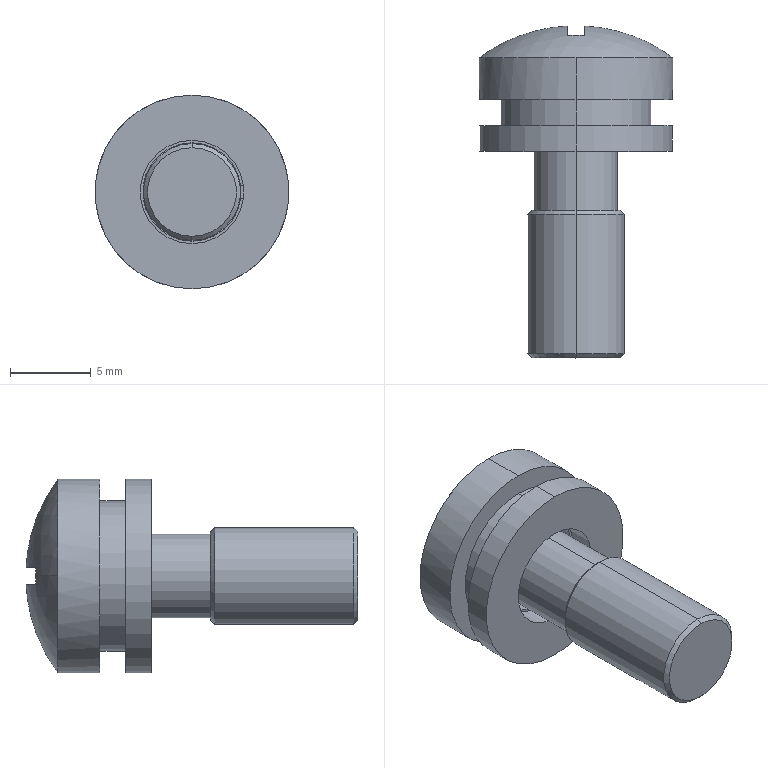Part | STEP file | 3 solids | 46 faces | box 12 x 20.569 x 12 mm | volume 958.317 mm3 | plane 22 | cylinder 16 | cone 4 | torus 2 | sphere 2 | commonest cylinder face diameters 12 x4 6.1 x3 9.3 x3 5.2 x2 6 x2 6.4 x2
STEP:
#1=CARTESIAN_POINT('',(0.,-20.6,-2.75));
#2=VERTEX_POINT('',#1);
#3=CARTESIAN_POINT('',(0.,-20.6,2.75));
#4=VERTEX_POINT('',#3);
#5=CARTESIAN_POINT('',(0.,-20.6,0.));
#6=DIRECTION('',(0.,-1.,0.));
#7=DIRECTION('',(0.,0.,1.));
#8=AXIS2_PLACEMENT_3D('',#5,#6,#7);
#9=CIRCLE('',#8,2.75);
#10=EDGE_CURVE('',#2,#4,#9,.T.);
#11=ORIENTED_EDGE('',*,*,#10,.F.);
#12=CARTESIAN_POINT('',(0.,-20.35,-3.));
#13=VERTEX_POINT('',#12);
#14=CARTESIAN_POINT('',(0.,-20.6,-2.75));
#15=DIRECTION('',(0.,0.7071,-0.7071));
#16=VECTOR('',#15,1000.);
#17=LINE('',#14,#16);
#18=EDGE_CURVE('',#2,#13,#17,.T.);
#19=ORIENTED_EDGE('',*,*,#18,.T.);
#20=CARTESIAN_POINT('',(0.,-20.35,3.));
#21=VERTEX_POINT('',#20);
#22=CARTESIAN_POINT('',(0.,-20.35,0.));
#23=DIRECTION('',(0.,1.,0.));
#24=DIRECTION('',(0.,0.,1.));
#25=AXIS2_PLACEMENT_3D('',#22,#23,#24);
#26=CIRCLE('',#25,3.);
#27=EDGE_CURVE('',#21,#13,#26,.T.);
#28=ORIENTED_EDGE('',*,*,#27,.F.);
#29=CARTESIAN_POINT('',(0.,-20.6,2.75));
#30=DIRECTION('',(0.,0.7071,0.7071));
#31=VECTOR('',#30,1000.);
#32=LINE('',#29,#31);
#33=EDGE_CURVE('',#4,#21,#32,.T.);
#34=ORIENTED_EDGE('',*,*,#33,.F.);
#35=EDGE_LOOP('',(#11,#19,#28,#34));
#36=FACE_OUTER_BOUND('',#35,.T.);
#37=CARTESIAN_POINT('',(0.,-20.6,0.));
#38=DIRECTION('',(0.,1.,0.));
#39=DIRECTION('',(0.,0.,1.));
#40=AXIS2_PLACEMENT_3D('',#37,#38,#39);
#41=CONICAL_SURFACE('',#40,2.75,0.7854);
#42=ADVANCED_FACE('',(#36),#41,.T.);
#43=CARTESIAN_POINT('',(0.,-11.46,2.75));
#44=VERTEX_POINT('',#43);
#45=CARTESIAN_POINT('',(0.,-11.46,-2.75));
#46=VERTEX_POINT('',#45);
#47=CARTESIAN_POINT('',(0.,-11.46,0.));
#48=DIRECTION('',(0.,1.,0.));
#49=DIRECTION('',(0.,0.,1.));
#50=AXIS2_PLACEMENT_3D('',#47,#48,#49);
#51=CIRCLE('',#50,2.75);
#52=EDGE_CURVE('',#44,#46,#51,.T.);
#53=ORIENTED_EDGE('',*,*,#52,.F.);
#54=CARTESIAN_POINT('',(0.,-11.71,3.));
#55=VERTEX_POINT('',#54);
#56=CARTESIAN_POINT('',(0.,-11.71,3.));
#57=DIRECTION('',(0.,-0.7071,0.7071));
#58=VECTOR('',#57,1000.);
#59=LINE('',#56,#58);
#60=EDGE_CURVE('',#44,#55,#59,.T.);
#61=ORIENTED_EDGE('',*,*,#60,.T.);
#62=CARTESIAN_POINT('',(0.,-11.71,-3.));
#63=VERTEX_POINT('',#62);
#64=CARTESIAN_POINT('',(0.,-11.71,0.));
#65=DIRECTION('',(0.,-1.,0.));
#66=DIRECTION('',(0.,0.,1.));
#67=AXIS2_PLACEMENT_3D('',#64,#65,#66);
#68=CIRCLE('',#67,3.);
#69=EDGE_CURVE('',#63,#55,#68,.T.);
#70=ORIENTED_EDGE('',*,*,#69,.F.);
#71=CARTESIAN_POINT('',(0.,-11.71,-3.));
#72=DIRECTION('',(0.,-0.7071,-0.7071));
#73=VECTOR('',#72,1000.);
#74=LINE('',#71,#73);
#75=EDGE_CURVE('',#46,#63,#74,.T.);
#76=ORIENTED_EDGE('',*,*,#75,.F.);
#77=EDGE_LOOP('',(#53,#61,#70,#76));
#78=FACE_OUTER_BOUND('',#77,.T.);
#79=CARTESIAN_POINT('',(0.,-11.71,0.));
#80=DIRECTION('',(0.,-1.,0.));
#81=DIRECTION('',(0.,0.,-1.));
#82=AXIS2_PLACEMENT_3D('',#79,#80,#81);
#83=CONICAL_SURFACE('',#82,3.,0.7854);
#84=ADVANCED_FACE('',(#78),#83,.T.);
#85=CARTESIAN_POINT('',(0.,-4.85,2.6));
#86=VERTEX_POINT('',#85);
#87=CARTESIAN_POINT('',(0.,-4.85,-2.6));
#88=VERTEX_POINT('',#87);
#89=CARTESIAN_POINT('',(0.,-4.85,0.));
#90=DIRECTION('',(0.,-1.,0.));
#91=DIRECTION('',(0.,0.,-1.));
#92=AXIS2_PLACEMENT_3D('',#89,#90,#91);
#93=CIRCLE('',#92,2.6);
#94=EDGE_CURVE('',#86,#88,#93,.T.);
#95=ORIENTED_EDGE('',*,*,#94,.F.);
#96=CARTESIAN_POINT('',(0.,-4.6,2.85));
#97=VERTEX_POINT('',#96);
#98=CARTESIAN_POINT('',(0.,-4.85,2.85));
#99=DIRECTION('',(1.,0.,0.));
#100=DIRECTION('',(0.,0.,-1.));
#101=AXIS2_PLACEMENT_3D('',#98,#99,#100);
#102=CIRCLE('',#101,0.25);
#103=EDGE_CURVE('',#86,#97,#102,.T.);
#104=ORIENTED_EDGE('',*,*,#103,.T.);
#105=CARTESIAN_POINT('',(0.,-4.6,-2.85));
#106=VERTEX_POINT('',#105);
#107=CARTESIAN_POINT('',(0.,-4.6,0.));
#108=DIRECTION('',(0.,1.,0.));
#109=DIRECTION('',(0.,0.,-1.));
#110=AXIS2_PLACEMENT_3D('',#107,#108,#109);
#111=CIRCLE('',#110,2.85);
#112=EDGE_CURVE('',#106,#97,#111,.T.);
#113=ORIENTED_EDGE('',*,*,#112,.F.);
#114=CARTESIAN_POINT('',(0.,-4.85,-2.85));
#115=DIRECTION('',(-1.,0.,0.));
#116=DIRECTION('',(0.,0.,1.));
#117=AXIS2_PLACEMENT_3D('',#114,#115,#116);
#118=CIRCLE('',#117,0.25);
#119=EDGE_CURVE('',#88,#106,#118,.T.);
#120=ORIENTED_EDGE('',*,*,#119,.F.);
#121=EDGE_LOOP('',(#95,#104,#113,#120));
#122=FACE_OUTER_BOUND('',#121,.T.);
#123=CARTESIAN_POINT('',(0.,-4.85,0.));
#124=DIRECTION('',(0.,-1.,0.));
#125=DIRECTION('',(0.,0.,-1.));
#126=AXIS2_PLACEMENT_3D('',#123,#124,#125);
#127=TOROIDAL_SURFACE('',#126,2.85,0.25);
#128=ADVANCED_FACE('',(#122),#127,.F.);
#129=CARTESIAN_POINT('',(-3.45,-0.614,0.));
#130=VERTEX_POINT('',#129);
#131=CARTESIAN_POINT('',(-3.45,-0.6304,0.555));
#132=VERTEX_POINT('',#131);
#133=CARTESIAN_POINT('',(-3.45,-10.,0.));
#134=DIRECTION('',(1.,0.,0.));
#135=DIRECTION('',(0.,0.,1.));
#136=AXIS2_PLACEMENT_3D('',#133,#134,#135);
#137=CIRCLE('',#136,9.386);
#138=EDGE_CURVE('',#130,#132,#137,.T.);
#139=ORIENTED_EDGE('',*,*,#138,.F.);
#140=CARTESIAN_POINT('',(-6.,-2.,0.));
#141=VERTEX_POINT('',#140);
#142=CARTESIAN_POINT('',(0.,-10.,0.));
#143=DIRECTION('',(0.,0.,1.));
#144=DIRECTION('',(1.,0.,0.));
#145=AXIS2_PLACEMENT_3D('',#142,#143,#144);
#146=CIRCLE('',#145,10.);
#147=EDGE_CURVE('',#130,#141,#146,.T.);
#148=ORIENTED_EDGE('',*,*,#147,.T.);
#149=CARTESIAN_POINT('',(0.,-2.,6.));
#150=VERTEX_POINT('',#149);
#151=CARTESIAN_POINT('',(0.,-2.,0.));
#152=DIRECTION('',(0.,-1.,0.));
#153=DIRECTION('',(0.,0.,-1.));
#154=AXIS2_PLACEMENT_3D('',#151,#152,#153);
#155=CIRCLE('',#154,6.);
#156=EDGE_CURVE('',#150,#141,#155,.T.);
#157=ORIENTED_EDGE('',*,*,#156,.F.);
#158=CARTESIAN_POINT('',(6.,-2.,0.));
#159=VERTEX_POINT('',#158);
#160=CARTESIAN_POINT('',(0.,-2.,0.));
#161=DIRECTION('',(0.,-1.,0.));
#162=DIRECTION('',(0.,0.,-1.));
#163=AXIS2_PLACEMENT_3D('',#160,#161,#162);
#164=CIRCLE('',#163,6.);
#165=EDGE_CURVE('',#159,#150,#164,.T.);
#166=ORIENTED_EDGE('',*,*,#165,.F.);
#167=CARTESIAN_POINT('',(3.45,-0.614,0.));
#168=VERTEX_POINT('',#167);
#169=CARTESIAN_POINT('',(0.,-10.,0.));
#170=DIRECTION('',(0.,0.,-1.));
#171=DIRECTION('',(-1.,0.,0.));
#172=AXIS2_PLACEMENT_3D('',#169,#170,#171);
#173=CIRCLE('',#172,10.);
#174=EDGE_CURVE('',#168,#159,#173,.T.);
#175=ORIENTED_EDGE('',*,*,#174,.F.);
#176=CARTESIAN_POINT('',(3.45,-0.6304,0.555));
#177=VERTEX_POINT('',#176);
#178=CARTESIAN_POINT('',(3.45,-10.,0.));
#179=DIRECTION('',(-1.,0.,0.));
#180=DIRECTION('',(0.,0.,-1.));
#181=AXIS2_PLACEMENT_3D('',#178,#179,#180);
#182=CIRCLE('',#181,9.386);
#183=EDGE_CURVE('',#177,#168,#182,.T.);
#184=ORIENTED_EDGE('',*,*,#183,.F.);
#185=CARTESIAN_POINT('',(0.555,-0.03085,0.555));
#186=VERTEX_POINT('',#185);
#187=CARTESIAN_POINT('',(0.,-10.,0.555));
#188=DIRECTION('',(0.,0.,-1.));
#189=DIRECTION('',(1.,0.,0.));
#190=AXIS2_PLACEMENT_3D('',#187,#188,#189);
#191=CIRCLE('',#190,9.985);
#192=EDGE_CURVE('',#186,#177,#191,.T.);
#193=ORIENTED_EDGE('',*,*,#192,.F.);
#194=CARTESIAN_POINT('',(0.555,-0.6304,3.45));
#195=VERTEX_POINT('',#194);
#196=CARTESIAN_POINT('',(0.555,-10.,0.));
#197=DIRECTION('',(-1.,0.,0.));
#198=DIRECTION('',(0.,0.,-1.));
#199=AXIS2_PLACEMENT_3D('',#196,#197,#198);
#200=CIRCLE('',#199,9.985);
#201=EDGE_CURVE('',#195,#186,#200,.T.);
#202=ORIENTED_EDGE('',*,*,#201,.F.);
#203=CARTESIAN_POINT('',(-0.555,-0.6304,3.45));
#204=VERTEX_POINT('',#203);
#205=CARTESIAN_POINT('',(0.,-10.,3.45));
#206=DIRECTION('',(0.,0.,-1.));
#207=DIRECTION('',(1.,0.,0.));
#208=AXIS2_PLACEMENT_3D('',#205,#206,#207);
#209=CIRCLE('',#208,9.386);
#210=EDGE_CURVE('',#204,#195,#209,.T.);
#211=ORIENTED_EDGE('',*,*,#210,.F.);
#212=CARTESIAN_POINT('',(-0.555,-0.03085,0.555));
#213=VERTEX_POINT('',#212);
#214=CARTESIAN_POINT('',(-0.555,-10.,0.));
#215=DIRECTION('',(1.,0.,0.));
#216=DIRECTION('',(0.,0.,1.));
#217=AXIS2_PLACEMENT_3D('',#214,#215,#216);
#218=CIRCLE('',#217,9.985);
#219=EDGE_CURVE('',#213,#204,#218,.T.);
#220=ORIENTED_EDGE('',*,*,#219,.F.);
#221=CARTESIAN_POINT('',(0.,-10.,0.555));
#222=DIRECTION('',(0.,0.,-1.));
#223=DIRECTION('',(1.,0.,0.));
#224=AXIS2_PLACEMENT_3D('',#221,#222,#223);
#225=CIRCLE('',#224,9.985);
#226=EDGE_CURVE('',#132,#213,#225,.T.);
#227=ORIENTED_EDGE('',*,*,#226,.F.);
#228=EDGE_LOOP('',(#139,#148,#157,#166,#175,#184,#193,#202,#211,#220,#227));
#229=FACE_OUTER_BOUND('',#228,.T.);
#230=CARTESIAN_POINT('',(0.,-10.,0.));
#231=DIRECTION('',(0.,0.,1.));
#232=DIRECTION('',(1.,0.,0.));
#233=AXIS2_PLACEMENT_3D('',#230,#231,#232);
#234=SPHERICAL_SURFACE('',#233,10.);
#235=ADVANCED_FACE('',(#229),#234,.T.);
#236=CARTESIAN_POINT('',(0.,-2.,-6.));
#237=VERTEX_POINT('',#236);
#238=CARTESIAN_POINT('',(0.,-2.,0.));
#239=DIRECTION('',(0.,-1.,0.));
#240=DIRECTION('',(0.,0.,-1.));
#241=AXIS2_PLACEMENT_3D('',#238,#239,#240);
#242=CIRCLE('',#241,6.);
#243=EDGE_CURVE('',#237,#159,#242,.T.);
#244=ORIENTED_EDGE('',*,*,#243,.T.);
#245=ORIENTED_EDGE('',*,*,#165,.T.);
#246=CARTESIAN_POINT('',(0.,-4.6,6.));
#247=VERTEX_POINT('',#246);
#248=CARTESIAN_POINT('',(0.,-20.6,6.));
#249=DIRECTION('',(0.,-1.,0.));
#250=VECTOR('',#249,1000.);
#251=LINE('',#248,#250);
#252=EDGE_CURVE('',#150,#247,#251,.T.);
#253=ORIENTED_EDGE('',*,*,#252,.T.);
#254=CARTESIAN_POINT('',(0.,-4.6,-6.));
#255=VERTEX_POINT('',#254);
#256=CARTESIAN_POINT('',(0.,-4.6,0.));
#257=DIRECTION('',(0.,-1.,0.));
#258=DIRECTION('',(0.,0.,-1.));
#259=AXIS2_PLACEMENT_3D('',#256,#257,#258);
#260=CIRCLE('',#259,6.);
#261=EDGE_CURVE('',#255,#247,#260,.T.);
#262=ORIENTED_EDGE('',*,*,#261,.F.);
#263=CARTESIAN_POINT('',(0.,-20.6,-6.));
#264=DIRECTION('',(0.,-1.,0.));
#265=VECTOR('',#264,1000.);
#266=LINE('',#263,#265);
#267=EDGE_CURVE('',#237,#255,#266,.T.);
#268=ORIENTED_EDGE('',*,*,#267,.F.);
#269=EDGE_LOOP('',(#244,#245,#253,#262,#268));
#270=FACE_OUTER_BOUND('',#269,.T.);
#271=CARTESIAN_POINT('',(0.,-20.6,0.));
#272=DIRECTION('',(0.,-1.,0.));
#273=DIRECTION('',(0.,0.,-1.));
#274=AXIS2_PLACEMENT_3D('',#271,#272,#273);
#275=CYLINDRICAL_SURFACE('',#274,6.);
#276=ADVANCED_FACE('',(#270),#275,.T.);
#277=CARTESIAN_POINT('',(0.,-4.85,0.));
#278=DIRECTION('',(0.,-1.,0.));
#279=DIRECTION('',(0.,0.,-1.));
#280=AXIS2_PLACEMENT_3D('',#277,#278,#279);
#281=CIRCLE('',#280,2.6);
#282=EDGE_CURVE('',#88,#86,#281,.T.);
#283=ORIENTED_EDGE('',*,*,#282,.T.);
#284=CARTESIAN_POINT('',(0.,-11.46,2.6));
#285=VERTEX_POINT('',#284);
#286=CARTESIAN_POINT('',(0.,-20.6,2.6));
#287=DIRECTION('',(0.,-1.,0.));
#288=VECTOR('',#287,1000.);
#289=LINE('',#286,#288);
#290=EDGE_CURVE('',#86,#285,#289,.T.);
#291=ORIENTED_EDGE('',*,*,#290,.T.);
#292=CARTESIAN_POINT('',(0.,-11.46,-2.6));
#293=VERTEX_POINT('',#292);
#294=CARTESIAN_POINT('',(0.,-11.46,0.));
#295=DIRECTION('',(0.,-1.,0.));
#296=DIRECTION('',(0.,0.,-1.));
#297=AXIS2_PLACEMENT_3D('',#294,#295,#296);
#298=CIRCLE('',#297,2.6);
#299=EDGE_CURVE('',#293,#285,#298,.T.);
#300=ORIENTED_EDGE('',*,*,#299,.F.);
#301=CARTESIAN_POINT('',(0.,-20.6,-2.6));
#302=DIRECTION('',(0.,-1.,0.));
#303=VECTOR('',#302,1000.);
#304=LINE('',#301,#303);
#305=EDGE_CURVE('',#88,#293,#304,.T.);
#306=ORIENTED_EDGE('',*,*,#305,.F.);
#307=EDGE_LOOP('',(#283,#291,#300,#306));
#308=FACE_OUTER_BOUND('',#307,.T.);
#309=CARTESIAN_POINT('',(0.,-20.6,0.));
#310=DIRECTION('',(0.,-1.,0.));
#311=DIRECTION('',(0.,0.,-1.));
#312=AXIS2_PLACEMENT_3D('',#309,#310,#311);
#313=CYLINDRICAL_SURFACE('',#312,2.6);
#314=ADVANCED_FACE('',(#308),#313,.T.);
#315=ORIENTED_EDGE('',*,*,#69,.T.);
#316=CARTESIAN_POINT('',(0.,-20.6,3.));
#317=DIRECTION('',(0.,-1.,0.));
#318=VECTOR('',#317,1000.);
#319=LINE('',#316,#318);
#320=EDGE_CURVE('',#55,#21,#319,.T.);
#321=ORIENTED_EDGE('',*,*,#320,.T.);
#322=ORIENTED_EDGE('',*,*,#27,.T.);
#323=CARTESIAN_POINT('',(0.,-20.6,-3.));
#324=DIRECTION('',(0.,-1.,0.));
#325=VECTOR('',#324,1000.);
#326=LINE('',#323,#325);
#327=EDGE_CURVE('',#63,#13,#326,.T.);
#328=ORIENTED_EDGE('',*,*,#327,.F.);
#329=EDGE_LOOP('',(#315,#321,#322,#328));
#330=FACE_OUTER_BOUND('',#329,.T.);
#331=CARTESIAN_POINT('',(0.,-20.6,0.));
#332=DIRECTION('',(0.,-1.,0.));
#333=DIRECTION('',(0.,0.,-1.));
#334=AXIS2_PLACEMENT_3D('',#331,#332,#333);
#335=CYLINDRICAL_SURFACE('',#334,3.);
#336=ADVANCED_FACE('',(#330),#335,.T.);
#337=CARTESIAN_POINT('',(0.,-20.6,0.));
#338=DIRECTION('',(0.,-1.,0.));
#339=DIRECTION('',(0.,0.,1.));
#340=AXIS2_PLACEMENT_3D('',#337,#338,#339);
#341=CIRCLE('',#340,2.75);
#342=EDGE_CURVE('',#4,#2,#341,.T.);
#343=ORIENTED_EDGE('',*,*,#342,.T.);
#344=ORIENTED_EDGE('',*,*,#10,.T.);
#345=EDGE_LOOP('',(#343,#344));
#346=FACE_OUTER_BOUND('',#345,.T.);
#347=CARTESIAN_POINT('',(0.,-20.6,0.));
#348=DIRECTION('',(0.,1.,0.));
#349=DIRECTION('',(0.,0.,1.));
#350=AXIS2_PLACEMENT_3D('',#347,#348,#349);
#351=PLANE('',#350);
#352=ADVANCED_FACE('',(#346),#351,.F.);
#353=ORIENTED_EDGE('',*,*,#320,.F.);
#354=CARTESIAN_POINT('',(0.,-11.71,0.));
#355=DIRECTION('',(0.,-1.,0.));
#356=DIRECTION('',(0.,0.,1.));
#357=AXIS2_PLACEMENT_3D('',#354,#355,#356);
#358=CIRCLE('',#357,3.);
#359=EDGE_CURVE('',#55,#63,#358,.T.);
#360=ORIENTED_EDGE('',*,*,#359,.T.);
#361=ORIENTED_EDGE('',*,*,#327,.T.);
#362=CARTESIAN_POINT('',(0.,-20.35,0.));
#363=DIRECTION('',(0.,1.,0.));
#364=DIRECTION('',(0.,0.,1.));
#365=AXIS2_PLACEMENT_3D('',#362,#363,#364);
#366=CIRCLE('',#365,3.);
#367=EDGE_CURVE('',#13,#21,#366,.T.);
#368=ORIENTED_EDGE('',*,*,#367,.T.);
#369=EDGE_LOOP('',(#353,#360,#361,#368));
#370=FACE_OUTER_BOUND('',#369,.T.);
#371=CARTESIAN_POINT('',(0.,-20.6,0.));
#372=DIRECTION('',(0.,-1.,0.));
#373=DIRECTION('',(0.,0.,-1.));
#374=AXIS2_PLACEMENT_3D('',#371,#372,#373);
#375=CYLINDRICAL_SURFACE('',#374,3.);
#376=ADVANCED_FACE('',(#370),#375,.T.);
#377=CARTESIAN_POINT('',(0.,-11.46,0.));
#378=DIRECTION('',(0.,1.,0.));
#379=DIRECTION('',(0.,0.,1.));
#380=AXIS2_PLACEMENT_3D('',#377,#378,#379);
#381=CIRCLE('',#380,2.75);
#382=EDGE_CURVE('',#46,#44,#381,.T.);
#383=ORIENTED_EDGE('',*,*,#382,.T.);
#384=ORIENTED_EDGE('',*,*,#52,.T.);
#385=EDGE_LOOP('',(#383,#384));
#386=FACE_OUTER_BOUND('',#385,.T.);
#387=ORIENTED_EDGE('',*,*,#299,.T.);
#388=CARTESIAN_POINT('',(0.,-11.46,0.));
#389=DIRECTION('',(0.,-1.,0.));
#390=DIRECTION('',(0.,0.,-1.));
#391=AXIS2_PLACEMENT_3D('',#388,#389,#390);
#392=CIRCLE('',#391,2.6);
#393=EDGE_CURVE('',#285,#293,#392,.T.);
#394=ORIENTED_EDGE('',*,*,#393,.T.);
#395=EDGE_LOOP('',(#387,#394));
#396=FACE_BOUND('',#395,.T.);
#397=CARTESIAN_POINT('',(0.,-11.46,0.));
#398=DIRECTION('',(0.,1.,0.));
#399=DIRECTION('',(0.,0.,1.));
#400=AXIS2_PLACEMENT_3D('',#397,#398,#399);
#401=PLANE('',#400);
#402=ADVANCED_FACE('',(#386,#396),#401,.T.);
#403=ORIENTED_EDGE('',*,*,#290,.F.);
#404=ORIENTED_EDGE('',*,*,#94,.T.);
#405=ORIENTED_EDGE('',*,*,#305,.T.);
#406=ORIENTED_EDGE('',*,*,#393,.F.);
#407=EDGE_LOOP('',(#403,#404,#405,#406));
#408=FACE_OUTER_BOUND('',#407,.T.);
#409=CARTESIAN_POINT('',(0.,-20.6,0.));
#410=DIRECTION('',(0.,-1.,0.));
#411=DIRECTION('',(0.,0.,-1.));
#412=AXIS2_PLACEMENT_3D('',#409,#410,#411);
#413=CYLINDRICAL_SURFACE('',#412,2.6);
#414=ADVANCED_FACE('',(#408),#413,.T.);
#415=ORIENTED_EDGE('',*,*,#112,.T.);
#416=CARTESIAN_POINT('',(0.,-4.6,0.));
#417=DIRECTION('',(0.,1.,0.));
#418=DIRECTION('',(0.,0.,-1.));
#419=AXIS2_PLACEMENT_3D('',#416,#417,#418);
#420=CIRCLE('',#419,2.85);
#421=EDGE_CURVE('',#97,#106,#420,.T.);
#422=ORIENTED_EDGE('',*,*,#421,.T.);
#423=EDGE_LOOP('',(#415,#422));
#424=FACE_BOUND('',#423,.T.);
#425=ORIENTED_EDGE('',*,*,#261,.T.);
#426=CARTESIAN_POINT('',(0.,-4.6,0.));
#427=DIRECTION('',(0.,-1.,0.));
#428=DIRECTION('',(0.,0.,-1.));
#429=AXIS2_PLACEMENT_3D('',#426,#427,#428);
#430=CIRCLE('',#429,6.);
#431=EDGE_CURVE('',#247,#255,#430,.T.);
#432=ORIENTED_EDGE('',*,*,#431,.T.);
#433=EDGE_LOOP('',(#425,#432));
#434=FACE_OUTER_BOUND('',#433,.T.);
#435=CARTESIAN_POINT('',(0.,-4.6,0.));
#436=DIRECTION('',(0.,-1.,0.));
#437=DIRECTION('',(0.,0.,-1.));
#438=AXIS2_PLACEMENT_3D('',#435,#436,#437);
#439=PLANE('',#438);
#440=ADVANCED_FACE('',(#424,#434),#439,.T.);
#441=ORIENTED_EDGE('',*,*,#252,.F.);
#442=ORIENTED_EDGE('',*,*,#156,.T.);
#443=CARTESIAN_POINT('',(0.,-2.,0.));
#444=DIRECTION('',(0.,-1.,0.));
#445=DIRECTION('',(0.,0.,-1.));
#446=AXIS2_PLACEMENT_3D('',#443,#444,#445);
#447=CIRCLE('',#446,6.);
#448=EDGE_CURVE('',#141,#237,#447,.T.);
#449=ORIENTED_EDGE('',*,*,#448,.T.);
#450=ORIENTED_EDGE('',*,*,#267,.T.);
#451=ORIENTED_EDGE('',*,*,#431,.F.);
#452=EDGE_LOOP('',(#441,#442,#449,#450,#451));
#453=FACE_OUTER_BOUND('',#452,.T.);
#454=CARTESIAN_POINT('',(0.,-20.6,0.));
#455=DIRECTION('',(0.,-1.,0.));
#456=DIRECTION('',(0.,0.,-1.));
#457=AXIS2_PLACEMENT_3D('',#454,#455,#456);
#458=CYLINDRICAL_SURFACE('',#457,6.);
#459=ADVANCED_FACE('',(#453),#458,.T.);
#460=ORIENTED_EDGE('',*,*,#147,.F.);
#461=CARTESIAN_POINT('',(-3.45,-0.6304,-0.555));
#462=VERTEX_POINT('',#461);
#463=CARTESIAN_POINT('',(-3.45,-10.,0.));
#464=DIRECTION('',(1.,0.,0.));
#465=DIRECTION('',(0.,0.,1.));
#466=AXIS2_PLACEMENT_3D('',#463,#464,#465);
#467=CIRCLE('',#466,9.386);
#468=EDGE_CURVE('',#462,#130,#467,.T.);
#469=ORIENTED_EDGE('',*,*,#468,.F.);
#470=CARTESIAN_POINT('',(-0.555,-0.03085,-0.555));
#471=VERTEX_POINT('',#470);
#472=CARTESIAN_POINT('',(0.,-10.,-0.555));
#473=DIRECTION('',(0.,0.,1.));
#474=DIRECTION('',(-1.,0.,0.));
#475=AXIS2_PLACEMENT_3D('',#472,#473,#474);
#476=CIRCLE('',#475,9.985);
#477=EDGE_CURVE('',#471,#462,#476,.T.);
#478=ORIENTED_EDGE('',*,*,#477,.F.);
#479=CARTESIAN_POINT('',(-0.555,-0.6304,-3.45));
#480=VERTEX_POINT('',#479);
#481=CARTESIAN_POINT('',(-0.555,-10.,0.));
#482=DIRECTION('',(1.,0.,0.));
#483=DIRECTION('',(0.,0.,1.));
#484=AXIS2_PLACEMENT_3D('',#481,#482,#483);
#485=CIRCLE('',#484,9.985);
#486=EDGE_CURVE('',#480,#471,#485,.T.);
#487=ORIENTED_EDGE('',*,*,#486,.F.);
#488=CARTESIAN_POINT('',(0.555,-0.6304,-3.45));
#489=VERTEX_POINT('',#488);
#490=CARTESIAN_POINT('',(0.,-10.,-3.45));
#491=DIRECTION('',(0.,0.,1.));
#492=DIRECTION('',(-1.,0.,0.));
#493=AXIS2_PLACEMENT_3D('',#490,#491,#492);
#494=CIRCLE('',#493,9.386);
#495=EDGE_CURVE('',#489,#480,#494,.T.);
#496=ORIENTED_EDGE('',*,*,#495,.F.);
#497=CARTESIAN_POINT('',(0.555,-0.03085,-0.555));
#498=VERTEX_POINT('',#497);
#499=CARTESIAN_POINT('',(0.555,-10.,0.));
#500=DIRECTION('',(-1.,0.,0.));
#501=DIRECTION('',(0.,0.,-1.));
#502=AXIS2_PLACEMENT_3D('',#499,#500,#501);
#503=CIRCLE('',#502,9.985);
#504=EDGE_CURVE('',#498,#489,#503,.T.);
#505=ORIENTED_EDGE('',*,*,#504,.F.);
#506=CARTESIAN_POINT('',(3.45,-0.6304,-0.555));
#507=VERTEX_POINT('',#506);
#508=CARTESIAN_POINT('',(0.,-10.,-0.555));
#509=DIRECTION('',(0.,0.,1.));
#510=DIRECTION('',(-1.,0.,0.));
#511=AXIS2_PLACEMENT_3D('',#508,#509,#510);
#512=CIRCLE('',#511,9.985);
#513=EDGE_CURVE('',#507,#498,#512,.T.);
#514=ORIENTED_EDGE('',*,*,#513,.F.);
#515=CARTESIAN_POINT('',(3.45,-10.,0.));
#516=DIRECTION('',(-1.,0.,0.));
#517=DIRECTION('',(0.,0.,-1.));
#518=AXIS2_PLACEMENT_3D('',#515,#516,#517);
#519=CIRCLE('',#518,9.386);
#520=EDGE_CURVE('',#168,#507,#519,.T.);
#521=ORIENTED_EDGE('',*,*,#520,.F.);
#522=ORIENTED_EDGE('',*,*,#174,.T.);
#523=ORIENTED_EDGE('',*,*,#243,.F.);
#524=ORIENTED_EDGE('',*,*,#448,.F.);
#525=EDGE_LOOP('',(#460,#469,#478,#487,#496,#505,#514,#521,#522,#523,#524));
#526=FACE_OUTER_BOUND('',#525,.T.);
#527=CARTESIAN_POINT('',(0.,-10.,0.));
#528=DIRECTION('',(0.,0.,1.));
#529=DIRECTION('',(1.,0.,0.));
#530=AXIS2_PLACEMENT_3D('',#527,#528,#529);
#531=SPHERICAL_SURFACE('',#530,10.);
#532=ADVANCED_FACE('',(#526),#531,.T.);
#533=ORIENTED_EDGE('',*,*,#513,.T.);
#534=CARTESIAN_POINT('',(0.555,-3.46,-0.555));
#535=VERTEX_POINT('',#534);
#536=CARTESIAN_POINT('',(0.555,-3.46,-0.555));
#537=DIRECTION('',(0.,1.,0.));
#538=VECTOR('',#537,1000.);
#539=LINE('',#536,#538);
#540=EDGE_CURVE('',#535,#498,#539,.T.);
#541=ORIENTED_EDGE('',*,*,#540,.F.);
#542=CARTESIAN_POINT('',(3.45,-3.46,-0.555));
#543=VERTEX_POINT('',#542);
#544=CARTESIAN_POINT('',(0.555,-3.46,-0.555));
#545=DIRECTION('',(-1.,0.,0.));
#546=VECTOR('',#545,1000.);
#547=LINE('',#544,#546);
#548=EDGE_CURVE('',#543,#535,#547,.T.);
#549=ORIENTED_EDGE('',*,*,#548,.F.);
#550=CARTESIAN_POINT('',(3.45,-3.46,-0.555));
#551=DIRECTION('',(0.,1.,0.));
#552=VECTOR('',#551,1000.);
#553=LINE('',#550,#552);
#554=EDGE_CURVE('',#543,#507,#553,.T.);
#555=ORIENTED_EDGE('',*,*,#554,.T.);
#556=EDGE_LOOP('',(#533,#541,#549,#555));
#557=FACE_OUTER_BOUND('',#556,.T.);
#558=CARTESIAN_POINT('',(0.555,-3.46,-0.555));
#559=DIRECTION('',(0.,0.,-1.));
#560=DIRECTION('',(-1.,0.,0.));
#561=AXIS2_PLACEMENT_3D('',#558,#559,#560);
#562=PLANE('',#561);
#563=ADVANCED_FACE('',(#557),#562,.F.);
#564=ORIENTED_EDGE('',*,*,#183,.T.);
#565=ORIENTED_EDGE('',*,*,#520,.T.);
#566=ORIENTED_EDGE('',*,*,#554,.F.);
#567=CARTESIAN_POINT('',(3.45,-3.46,0.555));
#568=VERTEX_POINT('',#567);
#569=CARTESIAN_POINT('',(3.45,-3.46,-0.555));
#570=DIRECTION('',(0.,0.,-1.));
#571=VECTOR('',#570,1000.);
#572=LINE('',#569,#571);
#573=EDGE_CURVE('',#568,#543,#572,.T.);
#574=ORIENTED_EDGE('',*,*,#573,.F.);
#575=CARTESIAN_POINT('',(3.45,-3.46,0.555));
#576=DIRECTION('',(0.,1.,0.));
#577=VECTOR('',#576,1000.);
#578=LINE('',#575,#577);
#579=EDGE_CURVE('',#568,#177,#578,.T.);
#580=ORIENTED_EDGE('',*,*,#579,.T.);
#581=EDGE_LOOP('',(#564,#565,#566,#574,#580));
#582=FACE_OUTER_BOUND('',#581,.T.);
#583=CARTESIAN_POINT('',(3.45,-3.46,-0.555));
#584=DIRECTION('',(1.,0.,0.));
#585=DIRECTION('',(0.,0.,-1.));
#586=AXIS2_PLACEMENT_3D('',#583,#584,#585);
#587=PLANE('',#586);
#588=ADVANCED_FACE('',(#582),#587,.F.);
#589=ORIENTED_EDGE('',*,*,#192,.T.);
#590=ORIENTED_EDGE('',*,*,#579,.F.);
#591=CARTESIAN_POINT('',(0.555,-3.46,0.555));
#592=VERTEX_POINT('',#591);
#593=CARTESIAN_POINT('',(0.555,-3.46,0.555));
#594=DIRECTION('',(1.,0.,0.));
#595=VECTOR('',#594,1000.);
#596=LINE('',#593,#595);
#597=EDGE_CURVE('',#592,#568,#596,.T.);
#598=ORIENTED_EDGE('',*,*,#597,.F.);
#599=CARTESIAN_POINT('',(0.555,-3.46,0.555));
#600=DIRECTION('',(0.,1.,0.));
#601=VECTOR('',#600,1000.);
#602=LINE('',#599,#601);
#603=EDGE_CURVE('',#592,#186,#602,.T.);
#604=ORIENTED_EDGE('',*,*,#603,.T.);
#605=EDGE_LOOP('',(#589,#590,#598,#604));
#606=FACE_OUTER_BOUND('',#605,.T.);
#607=CARTESIAN_POINT('',(0.555,-3.46,0.555));
#608=DIRECTION('',(0.,0.,1.));
#609=DIRECTION('',(1.,0.,0.));
#610=AXIS2_PLACEMENT_3D('',#607,#608,#609);
#611=PLANE('',#610);
#612=ADVANCED_FACE('',(#606),#611,.F.);
#613=ORIENTED_EDGE('',*,*,#201,.T.);
#614=ORIENTED_EDGE('',*,*,#603,.F.);
#615=CARTESIAN_POINT('',(0.555,-3.46,3.45));
#616=VERTEX_POINT('',#615);
#617=CARTESIAN_POINT('',(0.555,-3.46,3.45));
#618=DIRECTION('',(0.,0.,-1.));
#619=VECTOR('',#618,1000.);
#620=LINE('',#617,#619);
#621=EDGE_CURVE('',#616,#592,#620,.T.);
#622=ORIENTED_EDGE('',*,*,#621,.F.);
#623=CARTESIAN_POINT('',(0.555,-3.46,3.45));
#624=DIRECTION('',(0.,1.,0.));
#625=VECTOR('',#624,1000.);
#626=LINE('',#623,#625);
#627=EDGE_CURVE('',#616,#195,#626,.T.);
#628=ORIENTED_EDGE('',*,*,#627,.T.);
#629=EDGE_LOOP('',(#613,#614,#622,#628));
#630=FACE_OUTER_BOUND('',#629,.T.);
#631=CARTESIAN_POINT('',(0.555,-3.46,3.45));
#632=DIRECTION('',(1.,0.,0.));
#633=DIRECTION('',(0.,0.,-1.));
#634=AXIS2_PLACEMENT_3D('',#631,#632,#633);
#635=PLANE('',#634);
#636=ADVANCED_FACE('',(#630),#635,.F.);
#637=ORIENTED_EDGE('',*,*,#210,.T.);
#638=ORIENTED_EDGE('',*,*,#627,.F.);
#639=CARTESIAN_POINT('',(-0.555,-3.46,3.45));
#640=VERTEX_POINT('',#639);
#641=CARTESIAN_POINT('',(-0.555,-3.46,3.45));
#642=DIRECTION('',(1.,0.,0.));
#643=VECTOR('',#642,1000.);
#644=LINE('',#641,#643);
#645=EDGE_CURVE('',#640,#616,#644,.T.);
#646=ORIENTED_EDGE('',*,*,#645,.F.);
#647=CARTESIAN_POINT('',(-0.555,-3.46,3.45));
#648=DIRECTION('',(0.,1.,0.));
#649=VECTOR('',#648,1000.);
#650=LINE('',#647,#649);
#651=EDGE_CURVE('',#640,#204,#650,.T.);
#652=ORIENTED_EDGE('',*,*,#651,.T.);
#653=EDGE_LOOP('',(#637,#638,#646,#652));
#654=FACE_OUTER_BOUND('',#653,.T.);
#655=CARTESIAN_POINT('',(-0.555,-3.46,3.45));
#656=DIRECTION('',(0.,0.,1.));
#657=DIRECTION('',(1.,0.,0.));
#658=AXIS2_PLACEMENT_3D('',#655,#656,#657);
#659=PLANE('',#658);
#660=ADVANCED_FACE('',(#654),#659,.F.);
#661=ORIENTED_EDGE('',*,*,#219,.T.);
#662=ORIENTED_EDGE('',*,*,#651,.F.);
#663=CARTESIAN_POINT('',(-0.555,-3.46,0.555));
#664=VERTEX_POINT('',#663);
#665=CARTESIAN_POINT('',(-0.555,-3.46,3.45));
#666=DIRECTION('',(0.,0.,1.));
#667=VECTOR('',#666,1000.);
#668=LINE('',#665,#667);
#669=EDGE_CURVE('',#664,#640,#668,.T.);
#670=ORIENTED_EDGE('',*,*,#669,.F.);
#671=CARTESIAN_POINT('',(-0.555,-3.46,0.555));
#672=DIRECTION('',(0.,1.,0.));
#673=VECTOR('',#672,1000.);
#674=LINE('',#671,#673);
#675=EDGE_CURVE('',#664,#213,#674,.T.);
#676=ORIENTED_EDGE('',*,*,#675,.T.);
#677=EDGE_LOOP('',(#661,#662,#670,#676));
#678=FACE_OUTER_BOUND('',#677,.T.);
#679=CARTESIAN_POINT('',(-0.555,-3.46,3.45));
#680=DIRECTION('',(-1.,0.,0.));
#681=DIRECTION('',(0.,0.,1.));
#682=AXIS2_PLACEMENT_3D('',#679,#680,#681);
#683=PLANE('',#682);
#684=ADVANCED_FACE('',(#678),#683,.F.);
#685=ORIENTED_EDGE('',*,*,#226,.T.);
#686=ORIENTED_EDGE('',*,*,#675,.F.);
#687=CARTESIAN_POINT('',(-3.45,-3.46,0.555));
#688=VERTEX_POINT('',#687);
#689=CARTESIAN_POINT('',(-0.555,-3.46,0.555));
#690=DIRECTION('',(1.,0.,0.));
#691=VECTOR('',#690,1000.);
#692=LINE('',#689,#691);
#693=EDGE_CURVE('',#688,#664,#692,.T.);
#694=ORIENTED_EDGE('',*,*,#693,.F.);
#695=CARTESIAN_POINT('',(-3.45,-3.46,0.555));
#696=DIRECTION('',(0.,1.,0.));
#697=VECTOR('',#696,1000.);
#698=LINE('',#695,#697);
#699=EDGE_CURVE('',#688,#132,#698,.T.);
#700=ORIENTED_EDGE('',*,*,#699,.T.);
#701=EDGE_LOOP('',(#685,#686,#694,#700));
#702=FACE_OUTER_BOUND('',#701,.T.);
#703=CARTESIAN_POINT('',(-0.555,-3.46,0.555));
#704=DIRECTION('',(0.,0.,1.));
#705=DIRECTION('',(1.,0.,0.));
#706=AXIS2_PLACEMENT_3D('',#703,#704,#705);
#707=PLANE('',#706);
#708=ADVANCED_FACE('',(#702),#707,.F.);
#709=ORIENTED_EDGE('',*,*,#468,.T.);
#710=ORIENTED_EDGE('',*,*,#138,.T.);
#711=ORIENTED_EDGE('',*,*,#699,.F.);
#712=CARTESIAN_POINT('',(-3.45,-3.46,-0.555));
#713=VERTEX_POINT('',#712);
#714=CARTESIAN_POINT('',(-3.45,-3.46,-0.555));
#715=DIRECTION('',(0.,0.,1.));
#716=VECTOR('',#715,1000.);
#717=LINE('',#714,#716);
#718=EDGE_CURVE('',#713,#688,#717,.T.);
#719=ORIENTED_EDGE('',*,*,#718,.F.);
#720=CARTESIAN_POINT('',(-3.45,-3.46,-0.555));
#721=DIRECTION('',(0.,1.,0.));
#722=VECTOR('',#721,1000.);
#723=LINE('',#720,#722);
#724=EDGE_CURVE('',#713,#462,#723,.T.);
#725=ORIENTED_EDGE('',*,*,#724,.T.);
#726=EDGE_LOOP('',(#709,#710,#711,#719,#725));
#727=FACE_OUTER_BOUND('',#726,.T.);
#728=CARTESIAN_POINT('',(-3.45,-3.46,-0.555));
#729=DIRECTION('',(-1.,0.,0.));
#730=DIRECTION('',(0.,0.,1.));
#731=AXIS2_PLACEMENT_3D('',#728,#729,#730);
#732=PLANE('',#731);
#733=ADVANCED_FACE('',(#727),#732,.F.);
#734=ORIENTED_EDGE('',*,*,#477,.T.);
#735=ORIENTED_EDGE('',*,*,#724,.F.);
#736=CARTESIAN_POINT('',(-0.555,-3.46,-0.555));
#737=VERTEX_POINT('',#736);
#738=CARTESIAN_POINT('',(-0.555,-3.46,-0.555));
#739=DIRECTION('',(-1.,0.,0.));
#740=VECTOR('',#739,1000.);
#741=LINE('',#738,#740);
#742=EDGE_CURVE('',#737,#713,#741,.T.);
#743=ORIENTED_EDGE('',*,*,#742,.F.);
#744=CARTESIAN_POINT('',(-0.555,-3.46,-0.555));
#745=DIRECTION('',(0.,1.,0.));
#746=VECTOR('',#745,1000.);
#747=LINE('',#744,#746);
#748=EDGE_CURVE('',#737,#471,#747,.T.);
#749=ORIENTED_EDGE('',*,*,#748,.T.);
#750=EDGE_LOOP('',(#734,#735,#743,#749));
#751=FACE_OUTER_BOUND('',#750,.T.);
#752=CARTESIAN_POINT('',(-0.555,-3.46,-0.555));
#753=DIRECTION('',(0.,0.,-1.));
#754=DIRECTION('',(-1.,0.,0.));
#755=AXIS2_PLACEMENT_3D('',#752,#753,#754);
#756=PLANE('',#755);
#757=ADVANCED_FACE('',(#751),#756,.F.);
#758=ORIENTED_EDGE('',*,*,#486,.T.);
#759=ORIENTED_EDGE('',*,*,#748,.F.);
#760=CARTESIAN_POINT('',(-0.555,-3.46,-3.45));
#761=VERTEX_POINT('',#760);
#762=CARTESIAN_POINT('',(-0.555,-3.46,-3.45));
#763=DIRECTION('',(0.,0.,1.));
#764=VECTOR('',#763,1000.);
#765=LINE('',#762,#764);
#766=EDGE_CURVE('',#761,#737,#765,.T.);
#767=ORIENTED_EDGE('',*,*,#766,.F.);
#768=CARTESIAN_POINT('',(-0.555,-3.46,-3.45));
#769=DIRECTION('',(0.,1.,0.));
#770=VECTOR('',#769,1000.);
#771=LINE('',#768,#770);
#772=EDGE_CURVE('',#761,#480,#771,.T.);
#773=ORIENTED_EDGE('',*,*,#772,.T.);
#774=EDGE_LOOP('',(#758,#759,#767,#773));
#775=FACE_OUTER_BOUND('',#774,.T.);
#776=CARTESIAN_POINT('',(-0.555,-3.46,-3.45));
#777=DIRECTION('',(-1.,0.,0.));
#778=DIRECTION('',(0.,0.,1.));
#779=AXIS2_PLACEMENT_3D('',#776,#777,#778);
#780=PLANE('',#779);
#781=ADVANCED_FACE('',(#775),#780,.F.);
#782=ORIENTED_EDGE('',*,*,#495,.T.);
#783=ORIENTED_EDGE('',*,*,#772,.F.);
#784=CARTESIAN_POINT('',(0.555,-3.46,-3.45));
#785=VERTEX_POINT('',#784);
#786=CARTESIAN_POINT('',(-0.555,-3.46,-3.45));
#787=DIRECTION('',(-1.,0.,0.));
#788=VECTOR('',#787,1000.);
#789=LINE('',#786,#788);
#790=EDGE_CURVE('',#785,#761,#789,.T.);
#791=ORIENTED_EDGE('',*,*,#790,.F.);
#792=CARTESIAN_POINT('',(0.555,-3.46,-3.45));
#793=DIRECTION('',(0.,1.,0.));
#794=VECTOR('',#793,1000.);
#795=LINE('',#792,#794);
#796=EDGE_CURVE('',#785,#489,#795,.T.);
#797=ORIENTED_EDGE('',*,*,#796,.T.);
#798=EDGE_LOOP('',(#782,#783,#791,#797));
#799=FACE_OUTER_BOUND('',#798,.T.);
#800=CARTESIAN_POINT('',(-0.555,-3.46,-3.45));
#801=DIRECTION('',(0.,0.,-1.));
#802=DIRECTION('',(-1.,0.,0.));
#803=AXIS2_PLACEMENT_3D('',#800,#801,#802);
#804=PLANE('',#803);
#805=ADVANCED_FACE('',(#799),#804,.F.);
#806=ORIENTED_EDGE('',*,*,#504,.T.);
#807=ORIENTED_EDGE('',*,*,#796,.F.);
#808=CARTESIAN_POINT('',(0.555,-3.46,-3.45));
#809=DIRECTION('',(0.,0.,-1.));
#810=VECTOR('',#809,1000.);
#811=LINE('',#808,#810);
#812=EDGE_CURVE('',#535,#785,#811,.T.);
#813=ORIENTED_EDGE('',*,*,#812,.F.);
#814=ORIENTED_EDGE('',*,*,#540,.T.);
#815=EDGE_LOOP('',(#806,#807,#813,#814));
#816=FACE_OUTER_BOUND('',#815,.T.);
#817=CARTESIAN_POINT('',(0.555,-3.46,-3.45));
#818=DIRECTION('',(1.,0.,0.));
#819=DIRECTION('',(0.,0.,-1.));
#820=AXIS2_PLACEMENT_3D('',#817,#818,#819);
#821=PLANE('',#820);
#822=ADVANCED_FACE('',(#816),#821,.F.);
#823=ORIENTED_EDGE('',*,*,#548,.T.);
#824=ORIENTED_EDGE('',*,*,#812,.T.);
#825=ORIENTED_EDGE('',*,*,#790,.T.);
#826=ORIENTED_EDGE('',*,*,#766,.T.);
#827=ORIENTED_EDGE('',*,*,#742,.T.);
#828=ORIENTED_EDGE('',*,*,#718,.T.);
#829=ORIENTED_EDGE('',*,*,#693,.T.);
#830=ORIENTED_EDGE('',*,*,#669,.T.);
#831=ORIENTED_EDGE('',*,*,#645,.T.);
#832=ORIENTED_EDGE('',*,*,#621,.T.);
#833=ORIENTED_EDGE('',*,*,#597,.T.);
#834=ORIENTED_EDGE('',*,*,#573,.T.);
#835=EDGE_LOOP('',(#823,#824,#825,#826,#827,#828,#829,#830,#831,#832,#833,#834));
#836=FACE_OUTER_BOUND('',#835,.T.);
#837=CARTESIAN_POINT('',(0.,-3.46,0.));
#838=DIRECTION('',(0.,-1.,0.));
#839=DIRECTION('',(0.,0.,-1.));
#840=AXIS2_PLACEMENT_3D('',#837,#838,#839);
#841=PLANE('',#840);
#842=ADVANCED_FACE('',(#836),#841,.F.);
#843=ORIENTED_EDGE('',*,*,#103,.F.);
#844=ORIENTED_EDGE('',*,*,#282,.F.);
#845=ORIENTED_EDGE('',*,*,#119,.T.);
#846=ORIENTED_EDGE('',*,*,#421,.F.);
#847=EDGE_LOOP('',(#843,#844,#845,#846));
#848=FACE_OUTER_BOUND('',#847,.T.);
#849=CARTESIAN_POINT('',(0.,-4.85,0.));
#850=DIRECTION('',(0.,-1.,0.));
#851=DIRECTION('',(0.,0.,-1.));
#852=AXIS2_PLACEMENT_3D('',#849,#850,#851);
#853=TOROIDAL_SURFACE('',#852,2.85,0.25);
#854=ADVANCED_FACE('',(#848),#853,.F.);
#855=ORIENTED_EDGE('',*,*,#60,.F.);
#856=ORIENTED_EDGE('',*,*,#382,.F.);
#857=ORIENTED_EDGE('',*,*,#75,.T.);
#858=ORIENTED_EDGE('',*,*,#359,.F.);
#859=EDGE_LOOP('',(#855,#856,#857,#858));
#860=FACE_OUTER_BOUND('',#859,.T.);
#861=CARTESIAN_POINT('',(0.,-11.71,0.));
#862=DIRECTION('',(0.,-1.,0.));
#863=DIRECTION('',(0.,0.,-1.));
#864=AXIS2_PLACEMENT_3D('',#861,#862,#863);
#865=CONICAL_SURFACE('',#864,3.,0.7854);
#866=ADVANCED_FACE('',(#860),#865,.T.);
#867=ORIENTED_EDGE('',*,*,#18,.F.);
#868=ORIENTED_EDGE('',*,*,#342,.F.);
#869=ORIENTED_EDGE('',*,*,#33,.T.);
#870=ORIENTED_EDGE('',*,*,#367,.F.);
#871=EDGE_LOOP('',(#867,#868,#869,#870));
#872=FACE_OUTER_BOUND('',#871,.T.);
#873=CARTESIAN_POINT('',(0.,-20.6,0.));
#874=DIRECTION('',(0.,1.,0.));
#875=DIRECTION('',(0.,0.,1.));
#876=AXIS2_PLACEMENT_3D('',#873,#874,#875);
#877=CONICAL_SURFACE('',#876,2.75,0.7854);
#878=ADVANCED_FACE('',(#872),#877,.T.);
#879=CLOSED_SHELL('',(#42,#84,#128,#235,#276,#314,#336,#352,#376,#402,#414,#440,#459,#532,#563,#588,#612,#636,#660,#684,#708,#733,#757,#781,#805,#822,#842,#854,#866,#878));
#880=MANIFOLD_SOLID_BREP('',#879);
#881=CARTESIAN_POINT('',(0.,-6.2,3.05));
#882=VERTEX_POINT('',#881);
#883=CARTESIAN_POINT('',(0.,-6.2,-3.05));
#884=VERTEX_POINT('',#883);
#885=CARTESIAN_POINT('',(0.,-6.2,0.));
#886=DIRECTION('',(0.,-1.,0.));
#887=DIRECTION('',(0.,0.,-1.));
#888=AXIS2_PLACEMENT_3D('',#885,#886,#887);
#889=CIRCLE('',#888,3.05);
#890=EDGE_CURVE('',#882,#884,#889,.T.);
#891=ORIENTED_EDGE('',*,*,#890,.T.);
#892=CARTESIAN_POINT('',(0.,-4.6,-3.05));
#893=VERTEX_POINT('',#892);
#894=CARTESIAN_POINT('',(0.,-6.2,-3.05));
#895=DIRECTION('',(0.,1.,0.));
#896=VECTOR('',#895,1000.);
#897=LINE('',#894,#896);
#898=EDGE_CURVE('',#884,#893,#897,.T.);
#899=ORIENTED_EDGE('',*,*,#898,.T.);
#900=CARTESIAN_POINT('',(0.,-4.6,3.05));
#901=VERTEX_POINT('',#900);
#902=CARTESIAN_POINT('',(0.,-4.6,0.));
#903=DIRECTION('',(0.,-1.,0.));
#904=DIRECTION('',(0.,0.,-1.));
#905=AXIS2_PLACEMENT_3D('',#902,#903,#904);
#906=CIRCLE('',#905,3.05);
#907=EDGE_CURVE('',#901,#893,#906,.T.);
#908=ORIENTED_EDGE('',*,*,#907,.F.);
#909=CARTESIAN_POINT('',(0.,-6.2,3.05));
#910=DIRECTION('',(0.,1.,0.));
#911=VECTOR('',#910,1000.);
#912=LINE('',#909,#911);
#913=EDGE_CURVE('',#882,#901,#912,.T.);
#914=ORIENTED_EDGE('',*,*,#913,.F.);
#915=EDGE_LOOP('',(#891,#899,#908,#914));
#916=FACE_OUTER_BOUND('',#915,.T.);
#917=CARTESIAN_POINT('',(0.,-6.2,0.));
#918=DIRECTION('',(0.,1.,0.));
#919=DIRECTION('',(0.,0.,1.));
#920=AXIS2_PLACEMENT_3D('',#917,#918,#919);
#921=CYLINDRICAL_SURFACE('',#920,3.05);
#922=ADVANCED_FACE('',(#916),#921,.F.);
#923=CARTESIAN_POINT('',(3.024,-6.2,0.4));
#924=VERTEX_POINT('',#923);
#925=CARTESIAN_POINT('',(0.,-6.2,0.));
#926=DIRECTION('',(0.,-1.,0.));
#927=DIRECTION('',(0.,0.,-1.));
#928=AXIS2_PLACEMENT_3D('',#925,#926,#927);
#929=CIRCLE('',#928,3.05);
#930=EDGE_CURVE('',#924,#882,#929,.T.);
#931=ORIENTED_EDGE('',*,*,#930,.T.);
#932=ORIENTED_EDGE('',*,*,#913,.T.);
#933=CARTESIAN_POINT('',(3.024,-4.6,0.4));
#934=VERTEX_POINT('',#933);
#935=CARTESIAN_POINT('',(0.,-4.6,0.));
#936=DIRECTION('',(0.,-1.,0.));
#937=DIRECTION('',(0.,0.,-1.));
#938=AXIS2_PLACEMENT_3D('',#935,#936,#937);
#939=CIRCLE('',#938,3.05);
#940=EDGE_CURVE('',#934,#901,#939,.T.);
#941=ORIENTED_EDGE('',*,*,#940,.F.);
#942=CARTESIAN_POINT('',(3.024,-6.2,0.4));
#943=DIRECTION('',(0.,1.,0.));
#944=VECTOR('',#943,1000.);
#945=LINE('',#942,#944);
#946=EDGE_CURVE('',#924,#934,#945,.T.);
#947=ORIENTED_EDGE('',*,*,#946,.F.);
#948=EDGE_LOOP('',(#931,#932,#941,#947));
#949=FACE_OUTER_BOUND('',#948,.T.);
#950=CARTESIAN_POINT('',(0.,-6.2,0.));
#951=DIRECTION('',(0.,1.,0.));
#952=DIRECTION('',(0.,0.,1.));
#953=AXIS2_PLACEMENT_3D('',#950,#951,#952);
#954=CYLINDRICAL_SURFACE('',#953,3.05);
#955=ADVANCED_FACE('',(#949),#954,.F.);
#956=CARTESIAN_POINT('',(0.,-6.2,-4.65));
#957=VERTEX_POINT('',#956);
#958=CARTESIAN_POINT('',(4.633,-6.2,-0.4));
#959=VERTEX_POINT('',#958);
#960=CARTESIAN_POINT('',(0.,-6.2,0.));
#961=DIRECTION('',(0.,-1.,0.));
#962=DIRECTION('',(0.,0.,-1.));
#963=AXIS2_PLACEMENT_3D('',#960,#961,#962);
#964=CIRCLE('',#963,4.65);
#965=EDGE_CURVE('',#957,#959,#964,.T.);
#966=ORIENTED_EDGE('',*,*,#965,.F.);
#967=CARTESIAN_POINT('',(0.,-4.6,-4.65));
#968=VERTEX_POINT('',#967);
#969=CARTESIAN_POINT('',(0.,-6.2,-4.65));
#970=DIRECTION('',(0.,1.,0.));
#971=VECTOR('',#970,1000.);
#972=LINE('',#969,#971);
#973=EDGE_CURVE('',#957,#968,#972,.T.);
#974=ORIENTED_EDGE('',*,*,#973,.T.);
#975=CARTESIAN_POINT('',(4.633,-4.6,-0.4));
#976=VERTEX_POINT('',#975);
#977=CARTESIAN_POINT('',(0.,-4.6,0.));
#978=DIRECTION('',(0.,-1.,0.));
#979=DIRECTION('',(0.,0.,-1.));
#980=AXIS2_PLACEMENT_3D('',#977,#978,#979);
#981=CIRCLE('',#980,4.65);
#982=EDGE_CURVE('',#968,#976,#981,.T.);
#983=ORIENTED_EDGE('',*,*,#982,.T.);
#984=CARTESIAN_POINT('',(4.633,-6.2,-0.4));
#985=DIRECTION('',(0.,-1.,0.));
#986=VECTOR('',#985,1000.);
#987=LINE('',#984,#986);
#988=EDGE_CURVE('',#976,#959,#987,.T.);
#989=ORIENTED_EDGE('',*,*,#988,.T.);
#990=EDGE_LOOP('',(#966,#974,#983,#989));
#991=FACE_OUTER_BOUND('',#990,.T.);
#992=CARTESIAN_POINT('',(0.,-6.2,0.));
#993=DIRECTION('',(0.,1.,0.));
#994=DIRECTION('',(0.,0.,1.));
#995=AXIS2_PLACEMENT_3D('',#992,#993,#994);
#996=CYLINDRICAL_SURFACE('',#995,4.65);
#997=ADVANCED_FACE('',(#991),#996,.T.);
#998=ORIENTED_EDGE('',*,*,#973,.F.);
#999=CARTESIAN_POINT('',(0.,-6.2,4.65));
#1000=VERTEX_POINT('',#999);
#1001=CARTESIAN_POINT('',(0.,-6.2,0.));
#1002=DIRECTION('',(0.,-1.,0.));
#1003=DIRECTION('',(0.,0.,-1.));
#1004=AXIS2_PLACEMENT_3D('',#1001,#1002,#1003);
#1005=CIRCLE('',#1004,4.65);
#1006=EDGE_CURVE('',#1000,#957,#1005,.T.);
#1007=ORIENTED_EDGE('',*,*,#1006,.F.);
#1008=CARTESIAN_POINT('',(0.,-4.6,4.65));
#1009=VERTEX_POINT('',#1008);
#1010=CARTESIAN_POINT('',(0.,-6.2,4.65));
#1011=DIRECTION('',(0.,1.,0.));
#1012=VECTOR('',#1011,1000.);
#1013=LINE('',#1010,#1012);
#1014=EDGE_CURVE('',#1000,#1009,#1013,.T.);
#1015=ORIENTED_EDGE('',*,*,#1014,.T.);
#1016=CARTESIAN_POINT('',(0.,-4.6,0.));
#1017=DIRECTION('',(0.,-1.,0.));
#1018=DIRECTION('',(0.,0.,-1.));
#1019=AXIS2_PLACEMENT_3D('',#1016,#1017,#1018);
#1020=CIRCLE('',#1019,4.65);
#1021=EDGE_CURVE('',#1009,#968,#1020,.T.);
#1022=ORIENTED_EDGE('',*,*,#1021,.T.);
#1023=EDGE_LOOP('',(#998,#1007,#1015,#1022));
#1024=FACE_OUTER_BOUND('',#1023,.T.);
#1025=CARTESIAN_POINT('',(0.,-6.2,0.));
#1026=DIRECTION('',(0.,1.,0.));
#1027=DIRECTION('',(0.,0.,1.));
#1028=AXIS2_PLACEMENT_3D('',#1025,#1026,#1027);
#1029=CYLINDRICAL_SURFACE('',#1028,4.65);
#1030=ADVANCED_FACE('',(#1024),#1029,.T.);
#1031=CARTESIAN_POINT('',(3.024,-6.2,-0.4));
#1032=VERTEX_POINT('',#1031);
#1033=CARTESIAN_POINT('',(0.,-6.2,-0.4));
#1034=DIRECTION('',(1.,0.,0.));
#1035=VECTOR('',#1034,1000.);
#1036=LINE('',#1033,#1035);
#1037=EDGE_CURVE('',#1032,#959,#1036,.T.);
#1038=ORIENTED_EDGE('',*,*,#1037,.F.);
#1039=CARTESIAN_POINT('',(0.,-6.2,0.));
#1040=DIRECTION('',(0.,-1.,0.));
#1041=DIRECTION('',(0.,0.,-1.));
#1042=AXIS2_PLACEMENT_3D('',#1039,#1040,#1041);
#1043=CIRCLE('',#1042,3.05);
#1044=EDGE_CURVE('',#884,#1032,#1043,.T.);
#1045=ORIENTED_EDGE('',*,*,#1044,.F.);
#1046=ORIENTED_EDGE('',*,*,#890,.F.);
#1047=ORIENTED_EDGE('',*,*,#930,.F.);
#1048=CARTESIAN_POINT('',(4.633,-6.2,0.4));
#1049=VERTEX_POINT('',#1048);
#1050=CARTESIAN_POINT('',(0.,-6.2,0.4));
#1051=DIRECTION('',(-1.,0.,0.));
#1052=VECTOR('',#1051,1000.);
#1053=LINE('',#1050,#1052);
#1054=EDGE_CURVE('',#1049,#924,#1053,.T.);
#1055=ORIENTED_EDGE('',*,*,#1054,.F.);
#1056=CARTESIAN_POINT('',(0.,-6.2,0.));
#1057=DIRECTION('',(0.,-1.,0.));
#1058=DIRECTION('',(0.,0.,-1.));
#1059=AXIS2_PLACEMENT_3D('',#1056,#1057,#1058);
#1060=CIRCLE('',#1059,4.65);
#1061=EDGE_CURVE('',#1049,#1000,#1060,.T.);
#1062=ORIENTED_EDGE('',*,*,#1061,.T.);
#1063=ORIENTED_EDGE('',*,*,#1006,.T.);
#1064=ORIENTED_EDGE('',*,*,#965,.T.);
#1065=EDGE_LOOP('',(#1038,#1045,#1046,#1047,#1055,#1062,#1063,#1064));
#1066=FACE_OUTER_BOUND('',#1065,.T.);
#1067=CARTESIAN_POINT('',(0.,-6.2,0.));
#1068=DIRECTION('',(0.,-1.,0.));
#1069=DIRECTION('',(0.,0.,-1.));
#1070=AXIS2_PLACEMENT_3D('',#1067,#1068,#1069);
#1071=PLANE('',#1070);
#1072=ADVANCED_FACE('',(#1066),#1071,.T.);
#1073=ORIENTED_EDGE('',*,*,#940,.T.);
#1074=ORIENTED_EDGE('',*,*,#907,.T.);
#1075=CARTESIAN_POINT('',(3.024,-4.6,-0.4));
#1076=VERTEX_POINT('',#1075);
#1077=CARTESIAN_POINT('',(0.,-4.6,0.));
#1078=DIRECTION('',(0.,-1.,0.));
#1079=DIRECTION('',(0.,0.,-1.));
#1080=AXIS2_PLACEMENT_3D('',#1077,#1078,#1079);
#1081=CIRCLE('',#1080,3.05);
#1082=EDGE_CURVE('',#893,#1076,#1081,.T.);
#1083=ORIENTED_EDGE('',*,*,#1082,.T.);
#1084=CARTESIAN_POINT('',(0.,-4.6,-0.4));
#1085=DIRECTION('',(1.,0.,0.));
#1086=VECTOR('',#1085,1000.);
#1087=LINE('',#1084,#1086);
#1088=EDGE_CURVE('',#1076,#976,#1087,.T.);
#1089=ORIENTED_EDGE('',*,*,#1088,.T.);
#1090=ORIENTED_EDGE('',*,*,#982,.F.);
#1091=ORIENTED_EDGE('',*,*,#1021,.F.);
#1092=CARTESIAN_POINT('',(4.633,-4.6,0.4));
#1093=VERTEX_POINT('',#1092);
#1094=CARTESIAN_POINT('',(0.,-4.6,0.));
#1095=DIRECTION('',(0.,-1.,0.));
#1096=DIRECTION('',(0.,0.,-1.));
#1097=AXIS2_PLACEMENT_3D('',#1094,#1095,#1096);
#1098=CIRCLE('',#1097,4.65);
#1099=EDGE_CURVE('',#1093,#1009,#1098,.T.);
#1100=ORIENTED_EDGE('',*,*,#1099,.F.);
#1101=CARTESIAN_POINT('',(0.,-4.6,0.4));
#1102=DIRECTION('',(-1.,0.,0.));
#1103=VECTOR('',#1102,1000.);
#1104=LINE('',#1101,#1103);
#1105=EDGE_CURVE('',#1093,#934,#1104,.T.);
#1106=ORIENTED_EDGE('',*,*,#1105,.T.);
#1107=EDGE_LOOP('',(#1073,#1074,#1083,#1089,#1090,#1091,#1100,#1106));
#1108=FACE_OUTER_BOUND('',#1107,.T.);
#1109=CARTESIAN_POINT('',(0.,-4.6,0.));
#1110=DIRECTION('',(0.,-1.,0.));
#1111=DIRECTION('',(0.,0.,-1.));
#1112=AXIS2_PLACEMENT_3D('',#1109,#1110,#1111);
#1113=PLANE('',#1112);
#1114=ADVANCED_FACE('',(#1108),#1113,.F.);
#1115=ORIENTED_EDGE('',*,*,#1014,.F.);
#1116=ORIENTED_EDGE('',*,*,#1061,.F.);
#1117=CARTESIAN_POINT('',(4.633,-6.2,0.4));
#1118=DIRECTION('',(0.,1.,0.));
#1119=VECTOR('',#1118,1000.);
#1120=LINE('',#1117,#1119);
#1121=EDGE_CURVE('',#1049,#1093,#1120,.T.);
#1122=ORIENTED_EDGE('',*,*,#1121,.T.);
#1123=ORIENTED_EDGE('',*,*,#1099,.T.);
#1124=EDGE_LOOP('',(#1115,#1116,#1122,#1123));
#1125=FACE_OUTER_BOUND('',#1124,.T.);
#1126=CARTESIAN_POINT('',(0.,-6.2,0.));
#1127=DIRECTION('',(0.,1.,0.));
#1128=DIRECTION('',(0.,0.,1.));
#1129=AXIS2_PLACEMENT_3D('',#1126,#1127,#1128);
#1130=CYLINDRICAL_SURFACE('',#1129,4.65);
#1131=ADVANCED_FACE('',(#1125),#1130,.T.);
#1132=ORIENTED_EDGE('',*,*,#898,.F.);
#1133=ORIENTED_EDGE('',*,*,#1044,.T.);
#1134=CARTESIAN_POINT('',(3.024,-6.2,-0.4));
#1135=DIRECTION('',(0.,-1.,0.));
#1136=VECTOR('',#1135,1000.);
#1137=LINE('',#1134,#1136);
#1138=EDGE_CURVE('',#1076,#1032,#1137,.T.);
#1139=ORIENTED_EDGE('',*,*,#1138,.F.);
#1140=ORIENTED_EDGE('',*,*,#1082,.F.);
#1141=EDGE_LOOP('',(#1132,#1133,#1139,#1140));
#1142=FACE_OUTER_BOUND('',#1141,.T.);
#1143=CARTESIAN_POINT('',(0.,-6.2,0.));
#1144=DIRECTION('',(0.,1.,0.));
#1145=DIRECTION('',(0.,0.,1.));
#1146=AXIS2_PLACEMENT_3D('',#1143,#1144,#1145);
#1147=CYLINDRICAL_SURFACE('',#1146,3.05);
#1148=ADVANCED_FACE('',(#1142),#1147,.F.);
#1149=ORIENTED_EDGE('',*,*,#1054,.T.);
#1150=ORIENTED_EDGE('',*,*,#946,.T.);
#1151=ORIENTED_EDGE('',*,*,#1105,.F.);
#1152=ORIENTED_EDGE('',*,*,#1121,.F.);
#1153=EDGE_LOOP('',(#1149,#1150,#1151,#1152));
#1154=FACE_OUTER_BOUND('',#1153,.T.);
#1155=CARTESIAN_POINT('',(0.,-0.03085,0.4));
#1156=DIRECTION('',(0.,0.,1.));
#1157=DIRECTION('',(1.,0.,0.));
#1158=AXIS2_PLACEMENT_3D('',#1155,#1156,#1157);
#1159=PLANE('',#1158);
#1160=ADVANCED_FACE('',(#1154),#1159,.F.);
#1161=ORIENTED_EDGE('',*,*,#1088,.F.);
#1162=ORIENTED_EDGE('',*,*,#1138,.T.);
#1163=ORIENTED_EDGE('',*,*,#1037,.T.);
#1164=ORIENTED_EDGE('',*,*,#988,.F.);
#1165=EDGE_LOOP('',(#1161,#1162,#1163,#1164));
#1166=FACE_OUTER_BOUND('',#1165,.T.);
#1167=CARTESIAN_POINT('',(0.,-0.03085,-0.4));
#1168=DIRECTION('',(0.,0.,-1.));
#1169=DIRECTION('',(-1.,0.,0.));
#1170=AXIS2_PLACEMENT_3D('',#1167,#1168,#1169);
#1171=PLANE('',#1170);
#1172=ADVANCED_FACE('',(#1166),#1171,.F.);
#1173=CLOSED_SHELL('',(#922,#955,#997,#1030,#1072,#1114,#1131,#1148,#1160,#1172));
#1174=MANIFOLD_SOLID_BREP('',#1173);
#1175=CARTESIAN_POINT('',(0.,-7.8,3.2));
#1176=VERTEX_POINT('',#1175);
#1177=CARTESIAN_POINT('',(0.,-7.8,-3.2));
#1178=VERTEX_POINT('',#1177);
#1179=CARTESIAN_POINT('',(0.,-7.8,0.));
#1180=DIRECTION('',(0.,-1.,0.));
#1181=DIRECTION('',(0.,0.,-1.));
#1182=AXIS2_PLACEMENT_3D('',#1179,#1180,#1181);
#1183=CIRCLE('',#1182,3.2);
#1184=EDGE_CURVE('',#1176,#1178,#1183,.T.);
#1185=ORIENTED_EDGE('',*,*,#1184,.T.);
#1186=CARTESIAN_POINT('',(0.,-6.2,-3.2));
#1187=VERTEX_POINT('',#1186);
#1188=CARTESIAN_POINT('',(0.,-7.8,-3.2));
#1189=DIRECTION('',(0.,1.,0.));
#1190=VECTOR('',#1189,1000.);
#1191=LINE('',#1188,#1190);
#1192=EDGE_CURVE('',#1178,#1187,#1191,.T.);
#1193=ORIENTED_EDGE('',*,*,#1192,.T.);
#1194=CARTESIAN_POINT('',(0.,-6.2,3.2));
#1195=VERTEX_POINT('',#1194);
#1196=CARTESIAN_POINT('',(0.,-6.2,0.));
#1197=DIRECTION('',(0.,-1.,0.));
#1198=DIRECTION('',(0.,0.,-1.));
#1199=AXIS2_PLACEMENT_3D('',#1196,#1197,#1198);
#1200=CIRCLE('',#1199,3.2);
#1201=EDGE_CURVE('',#1195,#1187,#1200,.T.);
#1202=ORIENTED_EDGE('',*,*,#1201,.F.);
#1203=CARTESIAN_POINT('',(0.,-7.8,3.2));
#1204=DIRECTION('',(0.,1.,0.));
#1205=VECTOR('',#1204,1000.);
#1206=LINE('',#1203,#1205);
#1207=EDGE_CURVE('',#1176,#1195,#1206,.T.);
#1208=ORIENTED_EDGE('',*,*,#1207,.F.);
#1209=EDGE_LOOP('',(#1185,#1193,#1202,#1208));
#1210=FACE_OUTER_BOUND('',#1209,.T.);
#1211=CARTESIAN_POINT('',(0.,-7.8,0.));
#1212=DIRECTION('',(0.,1.,0.));
#1213=DIRECTION('',(0.,0.,1.));
#1214=AXIS2_PLACEMENT_3D('',#1211,#1212,#1213);
#1215=CYLINDRICAL_SURFACE('',#1214,3.2);
#1216=ADVANCED_FACE('',(#1210),#1215,.F.);
#1217=CARTESIAN_POINT('',(0.,-7.8,-6.));
#1218=VERTEX_POINT('',#1217);
#1219=CARTESIAN_POINT('',(0.,-7.8,6.));
#1220=VERTEX_POINT('',#1219);
#1221=CARTESIAN_POINT('',(0.,-7.8,0.));
#1222=DIRECTION('',(0.,-1.,0.));
#1223=DIRECTION('',(0.,0.,-1.));
#1224=AXIS2_PLACEMENT_3D('',#1221,#1222,#1223);
#1225=CIRCLE('',#1224,6.);
#1226=EDGE_CURVE('',#1218,#1220,#1225,.T.);
#1227=ORIENTED_EDGE('',*,*,#1226,.F.);
#1228=CARTESIAN_POINT('',(0.,-6.2,-6.));
#1229=VERTEX_POINT('',#1228);
#1230=CARTESIAN_POINT('',(0.,-7.8,-6.));
#1231=DIRECTION('',(0.,1.,0.));
#1232=VECTOR('',#1231,1000.);
#1233=LINE('',#1230,#1232);
#1234=EDGE_CURVE('',#1218,#1229,#1233,.T.);
#1235=ORIENTED_EDGE('',*,*,#1234,.T.);
#1236=CARTESIAN_POINT('',(0.,-6.2,6.));
#1237=VERTEX_POINT('',#1236);
#1238=CARTESIAN_POINT('',(0.,-6.2,0.));
#1239=DIRECTION('',(0.,-1.,0.));
#1240=DIRECTION('',(0.,0.,-1.));
#1241=AXIS2_PLACEMENT_3D('',#1238,#1239,#1240);
#1242=CIRCLE('',#1241,6.);
#1243=EDGE_CURVE('',#1229,#1237,#1242,.T.);
#1244=ORIENTED_EDGE('',*,*,#1243,.T.);
#1245=CARTESIAN_POINT('',(0.,-7.8,6.));
#1246=DIRECTION('',(0.,1.,0.));
#1247=VECTOR('',#1246,1000.);
#1248=LINE('',#1245,#1247);
#1249=EDGE_CURVE('',#1220,#1237,#1248,.T.);
#1250=ORIENTED_EDGE('',*,*,#1249,.F.);
#1251=EDGE_LOOP('',(#1227,#1235,#1244,#1250));
#1252=FACE_OUTER_BOUND('',#1251,.T.);
#1253=CARTESIAN_POINT('',(0.,-7.8,0.));
#1254=DIRECTION('',(0.,1.,0.));
#1255=DIRECTION('',(0.,0.,1.));
#1256=AXIS2_PLACEMENT_3D('',#1253,#1254,#1255);
#1257=CYLINDRICAL_SURFACE('',#1256,6.);
#1258=ADVANCED_FACE('',(#1252),#1257,.T.);
#1259=CARTESIAN_POINT('',(0.,-7.8,0.));
#1260=DIRECTION('',(0.,-1.,0.));
#1261=DIRECTION('',(0.,0.,-1.));
#1262=AXIS2_PLACEMENT_3D('',#1259,#1260,#1261);
#1263=CIRCLE('',#1262,6.);
#1264=EDGE_CURVE('',#1220,#1218,#1263,.T.);
#1265=ORIENTED_EDGE('',*,*,#1264,.T.);
#1266=ORIENTED_EDGE('',*,*,#1226,.T.);
#1267=EDGE_LOOP('',(#1265,#1266));
#1268=FACE_OUTER_BOUND('',#1267,.T.);
#1269=ORIENTED_EDGE('',*,*,#1184,.F.);
#1270=CARTESIAN_POINT('',(0.,-7.8,0.));
#1271=DIRECTION('',(0.,-1.,0.));
#1272=DIRECTION('',(0.,0.,-1.));
#1273=AXIS2_PLACEMENT_3D('',#1270,#1271,#1272);
#1274=CIRCLE('',#1273,3.2);
#1275=EDGE_CURVE('',#1178,#1176,#1274,.T.);
#1276=ORIENTED_EDGE('',*,*,#1275,.F.);
#1277=EDGE_LOOP('',(#1269,#1276));
#1278=FACE_BOUND('',#1277,.T.);
#1279=CARTESIAN_POINT('',(0.,-7.8,0.));
#1280=DIRECTION('',(0.,-1.,0.));
#1281=DIRECTION('',(0.,0.,-1.));
#1282=AXIS2_PLACEMENT_3D('',#1279,#1280,#1281);
#1283=PLANE('',#1282);
#1284=ADVANCED_FACE('',(#1268,#1278),#1283,.T.);
#1285=CARTESIAN_POINT('',(0.,-6.2,0.));
#1286=DIRECTION('',(0.,-1.,0.));
#1287=DIRECTION('',(0.,0.,-1.));
#1288=AXIS2_PLACEMENT_3D('',#1285,#1286,#1287);
#1289=CIRCLE('',#1288,6.);
#1290=EDGE_CURVE('',#1237,#1229,#1289,.T.);
#1291=ORIENTED_EDGE('',*,*,#1290,.F.);
#1292=ORIENTED_EDGE('',*,*,#1243,.F.);
#1293=EDGE_LOOP('',(#1291,#1292));
#1294=FACE_OUTER_BOUND('',#1293,.T.);
#1295=ORIENTED_EDGE('',*,*,#1201,.T.);
#1296=CARTESIAN_POINT('',(0.,-6.2,0.));
#1297=DIRECTION('',(0.,-1.,0.));
#1298=DIRECTION('',(0.,0.,-1.));
#1299=AXIS2_PLACEMENT_3D('',#1296,#1297,#1298);
#1300=CIRCLE('',#1299,3.2);
#1301=EDGE_CURVE('',#1187,#1195,#1300,.T.);
#1302=ORIENTED_EDGE('',*,*,#1301,.T.);
#1303=EDGE_LOOP('',(#1295,#1302));
#1304=FACE_BOUND('',#1303,.T.);
#1305=CARTESIAN_POINT('',(0.,-6.2,0.));
#1306=DIRECTION('',(0.,-1.,0.));
#1307=DIRECTION('',(0.,0.,-1.));
#1308=AXIS2_PLACEMENT_3D('',#1305,#1306,#1307);
#1309=PLANE('',#1308);
#1310=ADVANCED_FACE('',(#1294,#1304),#1309,.F.);
#1311=ORIENTED_EDGE('',*,*,#1234,.F.);
#1312=ORIENTED_EDGE('',*,*,#1264,.F.);
#1313=ORIENTED_EDGE('',*,*,#1249,.T.);
#1314=ORIENTED_EDGE('',*,*,#1290,.T.);
#1315=EDGE_LOOP('',(#1311,#1312,#1313,#1314));
#1316=FACE_OUTER_BOUND('',#1315,.T.);
#1317=CARTESIAN_POINT('',(0.,-7.8,0.));
#1318=DIRECTION('',(0.,1.,0.));
#1319=DIRECTION('',(0.,0.,1.));
#1320=AXIS2_PLACEMENT_3D('',#1317,#1318,#1319);
#1321=CYLINDRICAL_SURFACE('',#1320,6.);
#1322=ADVANCED_FACE('',(#1316),#1321,.T.);
#1323=ORIENTED_EDGE('',*,*,#1192,.F.);
#1324=ORIENTED_EDGE('',*,*,#1275,.T.);
#1325=ORIENTED_EDGE('',*,*,#1207,.T.);
#1326=ORIENTED_EDGE('',*,*,#1301,.F.);
#1327=EDGE_LOOP('',(#1323,#1324,#1325,#1326));
#1328=FACE_OUTER_BOUND('',#1327,.T.);
#1329=CARTESIAN_POINT('',(0.,-7.8,0.));
#1330=DIRECTION('',(0.,1.,0.));
#1331=DIRECTION('',(0.,0.,1.));
#1332=AXIS2_PLACEMENT_3D('',#1329,#1330,#1331);
#1333=CYLINDRICAL_SURFACE('',#1332,3.2);
#1334=ADVANCED_FACE('',(#1328),#1333,.F.);
#1335=CLOSED_SHELL('',(#1216,#1258,#1284,#1310,#1322,#1334));
#1336=MANIFOLD_SOLID_BREP('',#1335);
#1337=CARTESIAN_POINT('',(0.,0.,0.));
#1338=DIRECTION('',(0.,0.,1.));
#1339=DIRECTION('',(1.,0.,0.));
#1340=AXIS2_PLACEMENT_3D('',#1337,#1338,#1339);
#1341=(LENGTH_UNIT()NAMED_UNIT(*)SI_UNIT(.MILLI.,.METRE.));
#1342=UNCERTAINTY_MEASURE_WITH_UNIT(LENGTH_MEASURE(0.00001),#1341,'','');
#1343=(NAMED_UNIT(*)PLANE_ANGLE_UNIT()SI_UNIT($,.RADIAN.));
#1344=(NAMED_UNIT(*)SI_UNIT($,.STERADIAN.)SOLID_ANGLE_UNIT());
#1345=(GEOMETRIC_REPRESENTATION_CONTEXT(3)GLOBAL_UNCERTAINTY_ASSIGNED_CONTEXT((#1342))GLOBAL_UNIT_ASSIGNED_CONTEXT((#1341,#1343,#1344))REPRESENTATION_CONTEXT('',''));
#1346=ADVANCED_BREP_SHAPE_REPRESENTATION('',(#880,#1174,#1336,#1340),#1345);